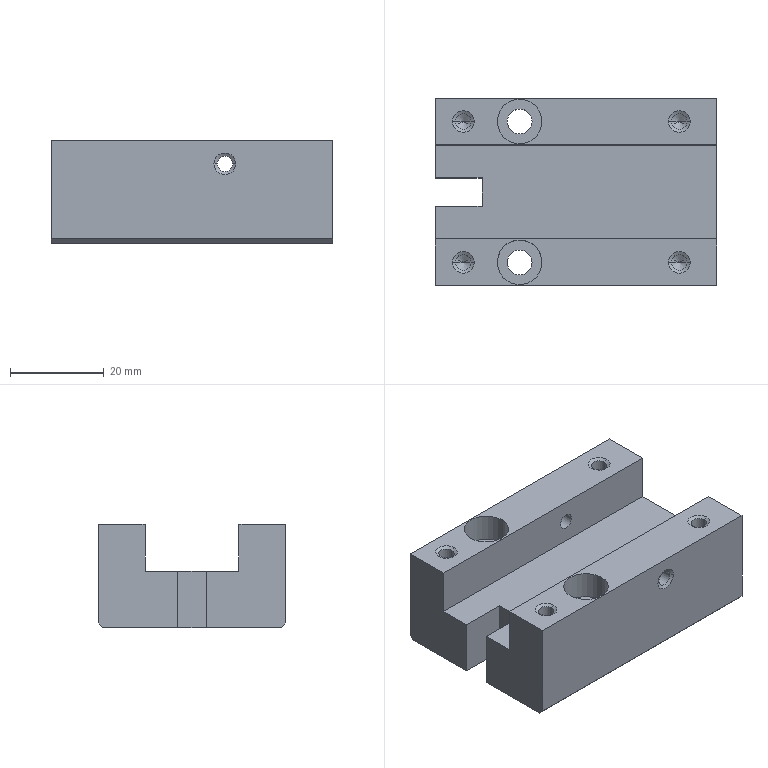Part | NX | 1 solid | 58 faces | box 60 x 40 x 22 mm | volume 37855 mm3 | cone 20 | cylinder 20 | plane 18 | commonest cylinder face diameters 3.3 x12 5.3 x4 9.5 x4